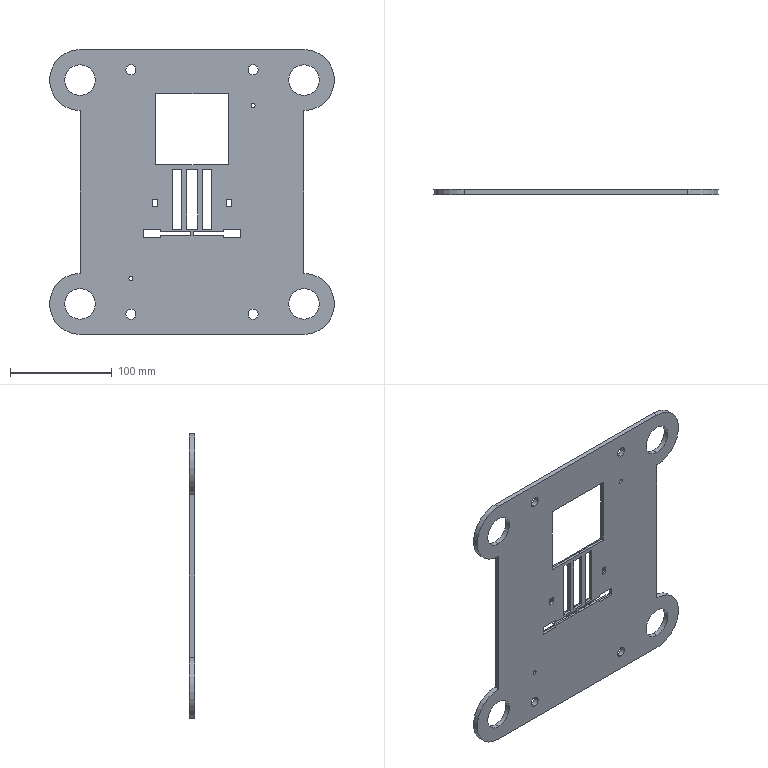Part | SolidWorks | features ICE 6, Extrusion 1 | 1 solid | 118 faces | box 280 x 5 x 280 mm | volume 281508 mm3 | plane 94 | cylinder 24 | commonest cylinder face diameters 10 x8 30 x8 4 x4 60 x4